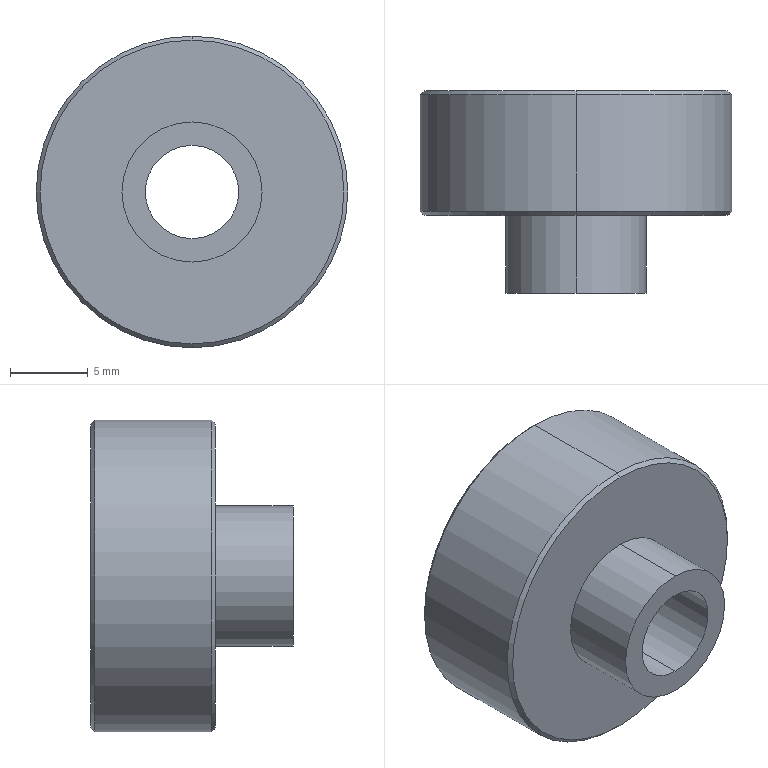Part | STEP file | BCC3 H14_12 | 1 solid | 13 faces | box 20 x 13 x 20 mm | volume 2460 mm3 | cylinder 6 | cone 4 | plane 3 | commonest cylinder face diameters 6 x2 9 x2 20 x2
STEP:
#1=CARTESIAN_POINT('',(0.,0.,0.));
#2=DIRECTION('',(0.,0.,1.));
#3=DIRECTION('',(1.,0.,0.));
#4=AXIS2_PLACEMENT_3D('',#1,#2,#3);
#5=CARTESIAN_POINT('',(0.,8.,9.75));
#6=VERTEX_POINT('',#5);
#7=CARTESIAN_POINT('',(0.,8.,-9.75));
#8=VERTEX_POINT('',#7);
#9=CARTESIAN_POINT('',(0.,8.,0.));
#10=DIRECTION('',(0.,1.,0.));
#11=DIRECTION('',(0.,0.,1.));
#12=AXIS2_PLACEMENT_3D('',#9,#10,#11);
#13=CIRCLE('',#12,9.75);
#14=CARTESIAN_POINT('',(0.,8.,0.));
#15=DIRECTION('',(0.,-1.,0.));
#16=DIRECTION('',(0.,0.,-1.));
#17=AXIS2_PLACEMENT_3D('',#14,#15,#16);
#18=CONICAL_SURFACE('',#17,9.75,0.7854);
#19=CARTESIAN_POINT('',(3.142,0.));
#20=DIRECTION('',(-1.,0.));
#21=VECTOR('',#20,1.);
#22=LINE('',#19,#21);
#23=(GEOMETRIC_REPRESENTATION_CONTEXT(2)PARAMETRIC_REPRESENTATION_CONTEXT()REPRESENTATION_CONTEXT('',''));
#24=DEFINITIONAL_REPRESENTATION('',(#22),#23);
#25=PCURVE('',#18,#24);
#26=CARTESIAN_POINT('',(0.,8.,0.));
#27=DIRECTION('',(0.,1.,0.));
#28=DIRECTION('',(0.,0.,1.));
#29=AXIS2_PLACEMENT_3D('',#26,#27,#28);
#30=PLANE('',#29);
#31=CARTESIAN_POINT('',(0.,0.));
#32=DIRECTION('',(1.,0.));
#33=AXIS2_PLACEMENT_2D('',#31,#32);
#34=CIRCLE('',#33,9.75);
#35=(GEOMETRIC_REPRESENTATION_CONTEXT(2)PARAMETRIC_REPRESENTATION_CONTEXT()REPRESENTATION_CONTEXT('',''));
#36=DEFINITIONAL_REPRESENTATION('',(#34),#35);
#37=PCURVE('',#30,#36);
#38=SURFACE_CURVE('',#13,(#25,#37),.PCURVE_S1.);
#39=EDGE_CURVE('',#6,#8,#38,.T.);
#40=ORIENTED_EDGE('',*,*,#39,.F.);
#41=CARTESIAN_POINT('',(0.,7.75,10.));
#42=VERTEX_POINT('',#41);
#43=CARTESIAN_POINT('',(0.,8.,9.75));
#44=DIRECTION('',(0.,-0.7071,0.7071));
#45=VECTOR('',#44,1.);
#46=LINE('',#43,#45);
#47=CARTESIAN_POINT('',(3.142,0.));
#48=DIRECTION('',(0.,1.));
#49=VECTOR('',#48,1.);
#50=LINE('',#47,#49);
#51=(GEOMETRIC_REPRESENTATION_CONTEXT(2)PARAMETRIC_REPRESENTATION_CONTEXT()REPRESENTATION_CONTEXT('',''));
#52=DEFINITIONAL_REPRESENTATION('',(#50),#51);
#53=PCURVE('',#18,#52);
#54=CARTESIAN_POINT('',(0.,8.,0.));
#55=DIRECTION('',(0.,-1.,0.));
#56=DIRECTION('',(0.,0.,-1.));
#57=AXIS2_PLACEMENT_3D('',#54,#55,#56);
#58=CONICAL_SURFACE('',#57,9.75,0.7854);
#59=CARTESIAN_POINT('',(3.142,0.));
#60=DIRECTION('',(0.,1.));
#61=VECTOR('',#60,1.);
#62=LINE('',#59,#61);
#63=(GEOMETRIC_REPRESENTATION_CONTEXT(2)PARAMETRIC_REPRESENTATION_CONTEXT()REPRESENTATION_CONTEXT('',''));
#64=DEFINITIONAL_REPRESENTATION('',(#62),#63);
#65=PCURVE('',#58,#64);
#66=SURFACE_CURVE('',#46,(#53,#65),.PCURVE_S1.);
#67=EDGE_CURVE('',#6,#42,#66,.T.);
#68=ORIENTED_EDGE('',*,*,#67,.T.);
#69=CARTESIAN_POINT('',(0.,7.75,-10.));
#70=VERTEX_POINT('',#69);
#71=CARTESIAN_POINT('',(0.,7.75,0.));
#72=DIRECTION('',(0.,-1.,0.));
#73=DIRECTION('',(0.,0.,1.));
#74=AXIS2_PLACEMENT_3D('',#71,#72,#73);
#75=CIRCLE('',#74,10.);
#76=CARTESIAN_POINT('',(-3.142,0.25));
#77=DIRECTION('',(1.,0.));
#78=VECTOR('',#77,1.);
#79=LINE('',#76,#78);
#80=(GEOMETRIC_REPRESENTATION_CONTEXT(2)PARAMETRIC_REPRESENTATION_CONTEXT()REPRESENTATION_CONTEXT('',''));
#81=DEFINITIONAL_REPRESENTATION('',(#79),#80);
#82=PCURVE('',#18,#81);
#83=CARTESIAN_POINT('',(0.,8.,0.));
#84=DIRECTION('',(0.,-1.,0.));
#85=DIRECTION('',(0.,0.,-1.));
#86=AXIS2_PLACEMENT_3D('',#83,#84,#85);
#87=CYLINDRICAL_SURFACE('',#86,10.);
#88=CARTESIAN_POINT('',(-3.142,0.25));
#89=DIRECTION('',(1.,0.));
#90=VECTOR('',#89,1.);
#91=LINE('',#88,#90);
#92=(GEOMETRIC_REPRESENTATION_CONTEXT(2)PARAMETRIC_REPRESENTATION_CONTEXT()REPRESENTATION_CONTEXT('',''));
#93=DEFINITIONAL_REPRESENTATION('',(#91),#92);
#94=PCURVE('',#87,#93);
#95=SURFACE_CURVE('',#75,(#82,#94),.PCURVE_S1.);
#96=EDGE_CURVE('',#70,#42,#95,.T.);
#97=ORIENTED_EDGE('',*,*,#96,.F.);
#98=CARTESIAN_POINT('',(0.,8.,-9.75));
#99=DIRECTION('',(0.,-0.7071,-0.7071));
#100=VECTOR('',#99,1.);
#101=LINE('',#98,#100);
#102=CARTESIAN_POINT('',(0.,0.));
#103=DIRECTION('',(0.,1.));
#104=VECTOR('',#103,1.);
#105=LINE('',#102,#104);
#106=(GEOMETRIC_REPRESENTATION_CONTEXT(2)PARAMETRIC_REPRESENTATION_CONTEXT()REPRESENTATION_CONTEXT('',''));
#107=DEFINITIONAL_REPRESENTATION('',(#105),#106);
#108=PCURVE('',#18,#107);
#109=CARTESIAN_POINT('',(6.283,0.));
#110=DIRECTION('',(0.,1.));
#111=VECTOR('',#110,1.);
#112=LINE('',#109,#111);
#113=(GEOMETRIC_REPRESENTATION_CONTEXT(2)PARAMETRIC_REPRESENTATION_CONTEXT()REPRESENTATION_CONTEXT('',''));
#114=DEFINITIONAL_REPRESENTATION('',(#112),#113);
#115=PCURVE('',#58,#114);
#116=SURFACE_CURVE('',#101,(#108,#115),.PCURVE_S1.);
#117=EDGE_CURVE('',#8,#70,#116,.T.);
#118=ORIENTED_EDGE('',*,*,#117,.F.);
#119=EDGE_LOOP('',(#40,#68,#97,#118));
#120=FACE_BOUND('',#119,.T.);
#121=ADVANCED_FACE('',(#120),#18,.T.);
#122=CARTESIAN_POINT('',(0.,0.,-9.75));
#123=VERTEX_POINT('',#122);
#124=CARTESIAN_POINT('',(0.,0.,9.75));
#125=VERTEX_POINT('',#124);
#126=CARTESIAN_POINT('',(0.,0.,0.));
#127=DIRECTION('',(0.,-1.,0.));
#128=DIRECTION('',(0.,0.,1.));
#129=AXIS2_PLACEMENT_3D('',#126,#127,#128);
#130=CIRCLE('',#129,9.75);
#131=CARTESIAN_POINT('',(0.,0.25,0.));
#132=DIRECTION('',(0.,1.,0.));
#133=DIRECTION('',(0.,0.,1.));
#134=AXIS2_PLACEMENT_3D('',#131,#132,#133);
#135=CONICAL_SURFACE('',#134,10.,0.7854);
#136=CARTESIAN_POINT('',(6.283,-0.25));
#137=DIRECTION('',(-1.,0.));
#138=VECTOR('',#137,1.);
#139=LINE('',#136,#138);
#140=(GEOMETRIC_REPRESENTATION_CONTEXT(2)PARAMETRIC_REPRESENTATION_CONTEXT()REPRESENTATION_CONTEXT('',''));
#141=DEFINITIONAL_REPRESENTATION('',(#139),#140);
#142=PCURVE('',#135,#141);
#143=CARTESIAN_POINT('',(0.,0.,0.));
#144=DIRECTION('',(0.,1.,0.));
#145=DIRECTION('',(0.,0.,1.));
#146=AXIS2_PLACEMENT_3D('',#143,#144,#145);
#147=PLANE('',#146);
#148=CARTESIAN_POINT('',(9.75,0.));
#149=CARTESIAN_POINT('',(9.75,-16.887));
#150=CARTESIAN_POINT('',(-4.875,-8.444));
#151=CARTESIAN_POINT('',(-19.5,0.));
#152=CARTESIAN_POINT('',(-4.875,8.444));
#153=CARTESIAN_POINT('',(9.75,16.887));
#154=CARTESIAN_POINT('',(9.75,0.));
#155=(BOUNDED_CURVE()B_SPLINE_CURVE(2,(#148,#149,#150,#151,#152,#153,#154),.UNSPECIFIED.,.T.,.F.)B_SPLINE_CURVE_WITH_KNOTS((1,2,2,2,2,1),(-2.094,0.,2.094,4.189,6.283,8.378),.UNSPECIFIED.)CURVE()GEOMETRIC_REPRESENTATION_ITEM()RATIONAL_B_SPLINE_CURVE((1.,0.5,1.,0.5,1.,0.5,1.))REPRESENTATION_ITEM(''));
#156=(GEOMETRIC_REPRESENTATION_CONTEXT(2)PARAMETRIC_REPRESENTATION_CONTEXT()REPRESENTATION_CONTEXT('',''));
#157=DEFINITIONAL_REPRESENTATION('',(#155),#156);
#158=PCURVE('',#147,#157);
#159=SURFACE_CURVE('',#130,(#142,#158),.PCURVE_S1.);
#160=EDGE_CURVE('',#123,#125,#159,.T.);
#161=ORIENTED_EDGE('',*,*,#160,.F.);
#162=CARTESIAN_POINT('',(0.,0.25,-10.));
#163=VERTEX_POINT('',#162);
#164=CARTESIAN_POINT('',(0.,0.25,-10.));
#165=DIRECTION('',(0.,0.7071,-0.7071));
#166=VECTOR('',#165,1.);
#167=LINE('',#164,#166);
#168=CARTESIAN_POINT('',(3.142,0.));
#169=DIRECTION('',(0.,1.));
#170=VECTOR('',#169,1.);
#171=LINE('',#168,#170);
#172=(GEOMETRIC_REPRESENTATION_CONTEXT(2)PARAMETRIC_REPRESENTATION_CONTEXT()REPRESENTATION_CONTEXT('',''));
#173=DEFINITIONAL_REPRESENTATION('',(#171),#172);
#174=PCURVE('',#135,#173);
#175=CARTESIAN_POINT('',(0.,0.25,0.));
#176=DIRECTION('',(0.,1.,0.));
#177=DIRECTION('',(0.,0.,1.));
#178=AXIS2_PLACEMENT_3D('',#175,#176,#177);
#179=CONICAL_SURFACE('',#178,10.,0.7854);
#180=CARTESIAN_POINT('',(3.142,0.));
#181=DIRECTION('',(0.,1.));
#182=VECTOR('',#181,1.);
#183=LINE('',#180,#182);
#184=(GEOMETRIC_REPRESENTATION_CONTEXT(2)PARAMETRIC_REPRESENTATION_CONTEXT()REPRESENTATION_CONTEXT('',''));
#185=DEFINITIONAL_REPRESENTATION('',(#183),#184);
#186=PCURVE('',#179,#185);
#187=SURFACE_CURVE('',#167,(#174,#186),.PCURVE_S1.);
#188=EDGE_CURVE('',#123,#163,#187,.T.);
#189=ORIENTED_EDGE('',*,*,#188,.T.);
#190=CARTESIAN_POINT('',(0.,0.25,10.));
#191=VERTEX_POINT('',#190);
#192=CARTESIAN_POINT('',(0.,0.25,0.));
#193=DIRECTION('',(0.,1.,0.));
#194=DIRECTION('',(0.,0.,1.));
#195=AXIS2_PLACEMENT_3D('',#192,#193,#194);
#196=CIRCLE('',#195,10.);
#197=CARTESIAN_POINT('',(0.,0.));
#198=DIRECTION('',(1.,0.));
#199=VECTOR('',#198,1.);
#200=LINE('',#197,#199);
#201=(GEOMETRIC_REPRESENTATION_CONTEXT(2)PARAMETRIC_REPRESENTATION_CONTEXT()REPRESENTATION_CONTEXT('',''));
#202=DEFINITIONAL_REPRESENTATION('',(#200),#201);
#203=PCURVE('',#135,#202);
#204=CARTESIAN_POINT('',(3.142,7.75));
#205=DIRECTION('',(-1.,0.));
#206=VECTOR('',#205,1.);
#207=LINE('',#204,#206);
#208=(GEOMETRIC_REPRESENTATION_CONTEXT(2)PARAMETRIC_REPRESENTATION_CONTEXT()REPRESENTATION_CONTEXT('',''));
#209=DEFINITIONAL_REPRESENTATION('',(#207),#208);
#210=PCURVE('',#87,#209);
#211=SURFACE_CURVE('',#196,(#203,#210),.PCURVE_S1.);
#212=EDGE_CURVE('',#191,#163,#211,.T.);
#213=ORIENTED_EDGE('',*,*,#212,.F.);
#214=CARTESIAN_POINT('',(0.,0.25,10.));
#215=DIRECTION('',(0.,0.7071,0.7071));
#216=VECTOR('',#215,1.);
#217=LINE('',#214,#216);
#218=CARTESIAN_POINT('',(0.,0.));
#219=DIRECTION('',(0.,1.));
#220=VECTOR('',#219,1.);
#221=LINE('',#218,#220);
#222=(GEOMETRIC_REPRESENTATION_CONTEXT(2)PARAMETRIC_REPRESENTATION_CONTEXT()REPRESENTATION_CONTEXT('',''));
#223=DEFINITIONAL_REPRESENTATION('',(#221),#222);
#224=PCURVE('',#135,#223);
#225=CARTESIAN_POINT('',(6.283,0.));
#226=DIRECTION('',(0.,1.));
#227=VECTOR('',#226,1.);
#228=LINE('',#225,#227);
#229=(GEOMETRIC_REPRESENTATION_CONTEXT(2)PARAMETRIC_REPRESENTATION_CONTEXT()REPRESENTATION_CONTEXT('',''));
#230=DEFINITIONAL_REPRESENTATION('',(#228),#229);
#231=PCURVE('',#179,#230);
#232=SURFACE_CURVE('',#217,(#224,#231),.PCURVE_S1.);
#233=EDGE_CURVE('',#125,#191,#232,.T.);
#234=ORIENTED_EDGE('',*,*,#233,.F.);
#235=EDGE_LOOP('',(#161,#189,#213,#234));
#236=FACE_BOUND('',#235,.T.);
#237=ADVANCED_FACE('',(#236),#135,.T.);
#238=CARTESIAN_POINT('',(0.,-5.,-4.5));
#239=VERTEX_POINT('',#238);
#240=CARTESIAN_POINT('',(0.,-5.,4.5));
#241=VERTEX_POINT('',#240);
#242=CARTESIAN_POINT('',(0.,-5.,0.));
#243=DIRECTION('',(0.,-1.,0.));
#244=DIRECTION('',(0.,0.,-1.));
#245=AXIS2_PLACEMENT_3D('',#242,#243,#244);
#246=CIRCLE('',#245,4.5);
#247=CARTESIAN_POINT('',(0.,-5.,0.));
#248=DIRECTION('',(0.,1.,0.));
#249=DIRECTION('',(0.,0.,1.));
#250=AXIS2_PLACEMENT_3D('',#247,#248,#249);
#251=CYLINDRICAL_SURFACE('',#250,4.5);
#252=CARTESIAN_POINT('',(3.142,0.));
#253=DIRECTION('',(-1.,0.));
#254=VECTOR('',#253,1.);
#255=LINE('',#252,#254);
#256=(GEOMETRIC_REPRESENTATION_CONTEXT(2)PARAMETRIC_REPRESENTATION_CONTEXT()REPRESENTATION_CONTEXT('',''));
#257=DEFINITIONAL_REPRESENTATION('',(#255),#256);
#258=PCURVE('',#251,#257);
#259=CARTESIAN_POINT('',(0.,-5.,0.));
#260=DIRECTION('',(0.,-1.,0.));
#261=DIRECTION('',(0.,0.,-1.));
#262=AXIS2_PLACEMENT_3D('',#259,#260,#261);
#263=PLANE('',#262);
#264=CARTESIAN_POINT('',(0.,0.));
#265=DIRECTION('',(1.,0.));
#266=AXIS2_PLACEMENT_2D('',#264,#265);
#267=CIRCLE('',#266,4.5);
#268=(GEOMETRIC_REPRESENTATION_CONTEXT(2)PARAMETRIC_REPRESENTATION_CONTEXT()REPRESENTATION_CONTEXT('',''));
#269=DEFINITIONAL_REPRESENTATION('',(#267),#268);
#270=PCURVE('',#263,#269);
#271=SURFACE_CURVE('',#246,(#258,#270),.PCURVE_S1.);
#272=EDGE_CURVE('',#239,#241,#271,.T.);
#273=ORIENTED_EDGE('',*,*,#272,.F.);
#274=CARTESIAN_POINT('',(0.,0.,-4.5));
#275=VERTEX_POINT('',#274);
#276=CARTESIAN_POINT('',(0.,-5.,-4.5));
#277=DIRECTION('',(0.,1.,0.));
#278=VECTOR('',#277,1.);
#279=LINE('',#276,#278);
#280=CARTESIAN_POINT('',(3.142,0.));
#281=DIRECTION('',(0.,1.));
#282=VECTOR('',#281,1.);
#283=LINE('',#280,#282);
#284=(GEOMETRIC_REPRESENTATION_CONTEXT(2)PARAMETRIC_REPRESENTATION_CONTEXT()REPRESENTATION_CONTEXT('',''));
#285=DEFINITIONAL_REPRESENTATION('',(#283),#284);
#286=PCURVE('',#251,#285);
#287=CARTESIAN_POINT('',(0.,-5.,0.));
#288=DIRECTION('',(0.,1.,0.));
#289=DIRECTION('',(0.,0.,1.));
#290=AXIS2_PLACEMENT_3D('',#287,#288,#289);
#291=CYLINDRICAL_SURFACE('',#290,4.5);
#292=CARTESIAN_POINT('',(3.142,0.));
#293=DIRECTION('',(0.,1.));
#294=VECTOR('',#293,1.);
#295=LINE('',#292,#294);
#296=(GEOMETRIC_REPRESENTATION_CONTEXT(2)PARAMETRIC_REPRESENTATION_CONTEXT()REPRESENTATION_CONTEXT('',''));
#297=DEFINITIONAL_REPRESENTATION('',(#295),#296);
#298=PCURVE('',#291,#297);
#299=SURFACE_CURVE('',#279,(#286,#298),.PCURVE_S1.);
#300=EDGE_CURVE('',#239,#275,#299,.T.);
#301=ORIENTED_EDGE('',*,*,#300,.T.);
#302=CARTESIAN_POINT('',(0.,0.,4.5));
#303=VERTEX_POINT('',#302);
#304=CARTESIAN_POINT('',(0.,0.,0.));
#305=DIRECTION('',(0.,-1.,0.));
#306=DIRECTION('',(0.,0.,1.));
#307=AXIS2_PLACEMENT_3D('',#304,#305,#306);
#308=CIRCLE('',#307,4.5);
#309=CARTESIAN_POINT('',(6.283,5.));
#310=DIRECTION('',(-1.,0.));
#311=VECTOR('',#310,1.);
#312=LINE('',#309,#311);
#313=(GEOMETRIC_REPRESENTATION_CONTEXT(2)PARAMETRIC_REPRESENTATION_CONTEXT()REPRESENTATION_CONTEXT('',''));
#314=DEFINITIONAL_REPRESENTATION('',(#312),#313);
#315=PCURVE('',#251,#314);
#316=CARTESIAN_POINT('',(4.5,0.));
#317=CARTESIAN_POINT('',(4.5,-7.794));
#318=CARTESIAN_POINT('',(-2.25,-3.897));
#319=CARTESIAN_POINT('',(-9.,0.));
#320=CARTESIAN_POINT('',(-2.25,3.897));
#321=CARTESIAN_POINT('',(4.5,7.794));
#322=CARTESIAN_POINT('',(4.5,0.));
#323=(BOUNDED_CURVE()B_SPLINE_CURVE(2,(#316,#317,#318,#319,#320,#321,#322),.UNSPECIFIED.,.T.,.F.)B_SPLINE_CURVE_WITH_KNOTS((1,2,2,2,2,1),(-2.094,0.,2.094,4.189,6.283,8.378),.UNSPECIFIED.)CURVE()GEOMETRIC_REPRESENTATION_ITEM()RATIONAL_B_SPLINE_CURVE((1.,0.5,1.,0.5,1.,0.5,1.))REPRESENTATION_ITEM(''));
#324=(GEOMETRIC_REPRESENTATION_CONTEXT(2)PARAMETRIC_REPRESENTATION_CONTEXT()REPRESENTATION_CONTEXT('',''));
#325=DEFINITIONAL_REPRESENTATION('',(#323),#324);
#326=PCURVE('',#147,#325);
#327=SURFACE_CURVE('',#308,(#315,#326),.PCURVE_S1.);
#328=EDGE_CURVE('',#275,#303,#327,.T.);
#329=ORIENTED_EDGE('',*,*,#328,.T.);
#330=CARTESIAN_POINT('',(0.,-5.,4.5));
#331=DIRECTION('',(0.,1.,0.));
#332=VECTOR('',#331,1.);
#333=LINE('',#330,#332);
#334=CARTESIAN_POINT('',(0.,0.));
#335=DIRECTION('',(0.,1.));
#336=VECTOR('',#335,1.);
#337=LINE('',#334,#336);
#338=(GEOMETRIC_REPRESENTATION_CONTEXT(2)PARAMETRIC_REPRESENTATION_CONTEXT()REPRESENTATION_CONTEXT('',''));
#339=DEFINITIONAL_REPRESENTATION('',(#337),#338);
#340=PCURVE('',#251,#339);
#341=CARTESIAN_POINT('',(6.283,0.));
#342=DIRECTION('',(0.,1.));
#343=VECTOR('',#342,1.);
#344=LINE('',#341,#343);
#345=(GEOMETRIC_REPRESENTATION_CONTEXT(2)PARAMETRIC_REPRESENTATION_CONTEXT()REPRESENTATION_CONTEXT('',''));
#346=DEFINITIONAL_REPRESENTATION('',(#344),#345);
#347=PCURVE('',#291,#346);
#348=SURFACE_CURVE('',#333,(#340,#347),.PCURVE_S1.);
#349=EDGE_CURVE('',#241,#303,#348,.T.);
#350=ORIENTED_EDGE('',*,*,#349,.F.);
#351=EDGE_LOOP('',(#273,#301,#329,#350));
#352=FACE_BOUND('',#351,.T.);
#353=ADVANCED_FACE('',(#352),#251,.T.);
#354=CARTESIAN_POINT('',(0.,8.,-3.));
#355=VERTEX_POINT('',#354);
#356=CARTESIAN_POINT('',(0.,-5.,-3.));
#357=VERTEX_POINT('',#356);
#358=CARTESIAN_POINT('',(0.,8.,-3.));
#359=DIRECTION('',(0.,-1.,0.));
#360=VECTOR('',#359,1.);
#361=LINE('',#358,#360);
#362=CARTESIAN_POINT('',(0.,8.,0.));
#363=DIRECTION('',(0.,-1.,0.));
#364=DIRECTION('',(0.,0.,-1.));
#365=AXIS2_PLACEMENT_3D('',#362,#363,#364);
#366=CYLINDRICAL_SURFACE('',#365,3.);
#367=CARTESIAN_POINT('',(6.283,0.));
#368=DIRECTION('',(0.,1.));
#369=VECTOR('',#368,1.);
#370=LINE('',#367,#369);
#371=(GEOMETRIC_REPRESENTATION_CONTEXT(2)PARAMETRIC_REPRESENTATION_CONTEXT()REPRESENTATION_CONTEXT('',''));
#372=DEFINITIONAL_REPRESENTATION('',(#370),#371);
#373=PCURVE('',#366,#372);
#374=CARTESIAN_POINT('',(0.,8.,0.));
#375=DIRECTION('',(0.,-1.,0.));
#376=DIRECTION('',(0.,0.,-1.));
#377=AXIS2_PLACEMENT_3D('',#374,#375,#376);
#378=CYLINDRICAL_SURFACE('',#377,3.);
#379=CARTESIAN_POINT('',(0.,0.));
#380=DIRECTION('',(0.,1.));
#381=VECTOR('',#380,1.);
#382=LINE('',#379,#381);
#383=(GEOMETRIC_REPRESENTATION_CONTEXT(2)PARAMETRIC_REPRESENTATION_CONTEXT()REPRESENTATION_CONTEXT('',''));
#384=DEFINITIONAL_REPRESENTATION('',(#382),#383);
#385=PCURVE('',#378,#384);
#386=SURFACE_CURVE('',#361,(#373,#385),.PCURVE_S1.);
#387=EDGE_CURVE('',#355,#357,#386,.T.);
#388=ORIENTED_EDGE('',*,*,#387,.T.);
#389=CARTESIAN_POINT('',(0.,-5.,3.));
#390=VERTEX_POINT('',#389);
#391=CARTESIAN_POINT('',(0.,-5.,0.));
#392=DIRECTION('',(0.,-1.,0.));
#393=DIRECTION('',(0.,0.,-1.));
#394=AXIS2_PLACEMENT_3D('',#391,#392,#393);
#395=CIRCLE('',#394,3.);
#396=CARTESIAN_POINT('',(0.,13.));
#397=DIRECTION('',(1.,0.));
#398=VECTOR('',#397,1.);
#399=LINE('',#396,#398);
#400=(GEOMETRIC_REPRESENTATION_CONTEXT(2)PARAMETRIC_REPRESENTATION_CONTEXT()REPRESENTATION_CONTEXT('',''));
#401=DEFINITIONAL_REPRESENTATION('',(#399),#400);
#402=PCURVE('',#366,#401);
#403=CARTESIAN_POINT('',(0.,0.));
#404=DIRECTION('',(1.,0.));
#405=AXIS2_PLACEMENT_2D('',#403,#404);
#406=CIRCLE('',#405,3.);
#407=(GEOMETRIC_REPRESENTATION_CONTEXT(2)PARAMETRIC_REPRESENTATION_CONTEXT()REPRESENTATION_CONTEXT('',''));
#408=DEFINITIONAL_REPRESENTATION('',(#406),#407);
#409=PCURVE('',#263,#408);
#410=SURFACE_CURVE('',#395,(#402,#409),.PCURVE_S1.);
#411=EDGE_CURVE('',#390,#357,#410,.T.);
#412=ORIENTED_EDGE('',*,*,#411,.F.);
#413=CARTESIAN_POINT('',(0.,8.,3.));
#414=VERTEX_POINT('',#413);
#415=CARTESIAN_POINT('',(0.,8.,3.));
#416=DIRECTION('',(0.,-1.,0.));
#417=VECTOR('',#416,1.);
#418=LINE('',#415,#417);
#419=CARTESIAN_POINT('',(3.142,0.));
#420=DIRECTION('',(0.,1.));
#421=VECTOR('',#420,1.);
#422=LINE('',#419,#421);
#423=(GEOMETRIC_REPRESENTATION_CONTEXT(2)PARAMETRIC_REPRESENTATION_CONTEXT()REPRESENTATION_CONTEXT('',''));
#424=DEFINITIONAL_REPRESENTATION('',(#422),#423);
#425=PCURVE('',#366,#424);
#426=CARTESIAN_POINT('',(3.142,0.));
#427=DIRECTION('',(0.,1.));
#428=VECTOR('',#427,1.);
#429=LINE('',#426,#428);
#430=(GEOMETRIC_REPRESENTATION_CONTEXT(2)PARAMETRIC_REPRESENTATION_CONTEXT()REPRESENTATION_CONTEXT('',''));
#431=DEFINITIONAL_REPRESENTATION('',(#429),#430);
#432=PCURVE('',#378,#431);
#433=SURFACE_CURVE('',#418,(#425,#432),.PCURVE_S1.);
#434=EDGE_CURVE('',#414,#390,#433,.T.);
#435=ORIENTED_EDGE('',*,*,#434,.F.);
#436=CARTESIAN_POINT('',(0.,8.,0.));
#437=DIRECTION('',(0.,1.,0.));
#438=DIRECTION('',(0.,0.,1.));
#439=AXIS2_PLACEMENT_3D('',#436,#437,#438);
#440=CIRCLE('',#439,3.);
#441=CARTESIAN_POINT('',(9.425,0.));
#442=DIRECTION('',(-1.,0.));
#443=VECTOR('',#442,1.);
#444=LINE('',#441,#443);
#445=(GEOMETRIC_REPRESENTATION_CONTEXT(2)PARAMETRIC_REPRESENTATION_CONTEXT()REPRESENTATION_CONTEXT('',''));
#446=DEFINITIONAL_REPRESENTATION('',(#444),#445);
#447=PCURVE('',#366,#446);
#448=CARTESIAN_POINT('',(0.,0.));
#449=DIRECTION('',(1.,0.));
#450=AXIS2_PLACEMENT_2D('',#448,#449);
#451=CIRCLE('',#450,3.);
#452=(GEOMETRIC_REPRESENTATION_CONTEXT(2)PARAMETRIC_REPRESENTATION_CONTEXT()REPRESENTATION_CONTEXT('',''));
#453=DEFINITIONAL_REPRESENTATION('',(#451),#452);
#454=PCURVE('',#30,#453);
#455=SURFACE_CURVE('',#440,(#447,#454),.PCURVE_S1.);
#456=EDGE_CURVE('',#355,#414,#455,.T.);
#457=ORIENTED_EDGE('',*,*,#456,.F.);
#458=EDGE_LOOP('',(#388,#412,#435,#457));
#459=FACE_BOUND('',#458,.F.);
#460=ADVANCED_FACE('',(#459),#366,.F.);
#461=ORIENTED_EDGE('',*,*,#96,.T.);
#462=CARTESIAN_POINT('',(0.,8.,10.));
#463=DIRECTION('',(0.,-1.,0.));
#464=VECTOR('',#463,1.);
#465=LINE('',#462,#464);
#466=CARTESIAN_POINT('',(3.142,0.));
#467=DIRECTION('',(0.,1.));
#468=VECTOR('',#467,1.);
#469=LINE('',#466,#468);
#470=(GEOMETRIC_REPRESENTATION_CONTEXT(2)PARAMETRIC_REPRESENTATION_CONTEXT()REPRESENTATION_CONTEXT('',''));
#471=DEFINITIONAL_REPRESENTATION('',(#469),#470);
#472=PCURVE('',#87,#471);
#473=CARTESIAN_POINT('',(0.,8.,0.));
#474=DIRECTION('',(0.,-1.,0.));
#475=DIRECTION('',(0.,0.,-1.));
#476=AXIS2_PLACEMENT_3D('',#473,#474,#475);
#477=CYLINDRICAL_SURFACE('',#476,10.);
#478=CARTESIAN_POINT('',(3.142,0.));
#479=DIRECTION('',(0.,1.));
#480=VECTOR('',#479,1.);
#481=LINE('',#478,#480);
#482=(GEOMETRIC_REPRESENTATION_CONTEXT(2)PARAMETRIC_REPRESENTATION_CONTEXT()REPRESENTATION_CONTEXT('',''));
#483=DEFINITIONAL_REPRESENTATION('',(#481),#482);
#484=PCURVE('',#477,#483);
#485=SURFACE_CURVE('',#465,(#472,#484),.PCURVE_S1.);
#486=EDGE_CURVE('',#42,#191,#485,.T.);
#487=ORIENTED_EDGE('',*,*,#486,.T.);
#488=ORIENTED_EDGE('',*,*,#212,.T.);
#489=CARTESIAN_POINT('',(0.,8.,-10.));
#490=DIRECTION('',(0.,-1.,0.));
#491=VECTOR('',#490,1.);
#492=LINE('',#489,#491);
#493=CARTESIAN_POINT('',(0.,0.));
#494=DIRECTION('',(0.,1.));
#495=VECTOR('',#494,1.);
#496=LINE('',#493,#495);
#497=(GEOMETRIC_REPRESENTATION_CONTEXT(2)PARAMETRIC_REPRESENTATION_CONTEXT()REPRESENTATION_CONTEXT('',''));
#498=DEFINITIONAL_REPRESENTATION('',(#496),#497);
#499=PCURVE('',#87,#498);
#500=CARTESIAN_POINT('',(6.283,0.));
#501=DIRECTION('',(0.,1.));
#502=VECTOR('',#501,1.);
#503=LINE('',#500,#502);
#504=(GEOMETRIC_REPRESENTATION_CONTEXT(2)PARAMETRIC_REPRESENTATION_CONTEXT()REPRESENTATION_CONTEXT('',''));
#505=DEFINITIONAL_REPRESENTATION('',(#503),#504);
#506=PCURVE('',#477,#505);
#507=SURFACE_CURVE('',#492,(#499,#506),.PCURVE_S1.);
#508=EDGE_CURVE('',#70,#163,#507,.T.);
#509=ORIENTED_EDGE('',*,*,#508,.F.);
#510=EDGE_LOOP('',(#461,#487,#488,#509));
#511=FACE_BOUND('',#510,.T.);
#512=ADVANCED_FACE('',(#511),#87,.T.);
#513=CARTESIAN_POINT('',(0.,0.,0.));
#514=DIRECTION('',(0.,-1.,0.));
#515=DIRECTION('',(0.,0.,1.));
#516=AXIS2_PLACEMENT_3D('',#513,#514,#515);
#517=CIRCLE('',#516,9.75);
#518=CARTESIAN_POINT('',(9.75,0.));
#519=CARTESIAN_POINT('',(9.75,-16.887));
#520=CARTESIAN_POINT('',(-4.875,-8.444));
#521=CARTESIAN_POINT('',(-19.5,0.));
#522=CARTESIAN_POINT('',(-4.875,8.444));
#523=CARTESIAN_POINT('',(9.75,16.887));
#524=CARTESIAN_POINT('',(9.75,0.));
#525=(BOUNDED_CURVE()B_SPLINE_CURVE(2,(#518,#519,#520,#521,#522,#523,#524),.UNSPECIFIED.,.T.,.F.)B_SPLINE_CURVE_WITH_KNOTS((1,2,2,2,2,1),(-2.094,0.,2.094,4.189,6.283,8.378),.UNSPECIFIED.)CURVE()GEOMETRIC_REPRESENTATION_ITEM()RATIONAL_B_SPLINE_CURVE((1.,0.5,1.,0.5,1.,0.5,1.))REPRESENTATION_ITEM(''));
#526=(GEOMETRIC_REPRESENTATION_CONTEXT(2)PARAMETRIC_REPRESENTATION_CONTEXT()REPRESENTATION_CONTEXT('',''));
#527=DEFINITIONAL_REPRESENTATION('',(#525),#526);
#528=PCURVE('',#147,#527);
#529=CARTESIAN_POINT('',(6.283,-0.25));
#530=DIRECTION('',(-1.,0.));
#531=VECTOR('',#530,1.);
#532=LINE('',#529,#531);
#533=(GEOMETRIC_REPRESENTATION_CONTEXT(2)PARAMETRIC_REPRESENTATION_CONTEXT()REPRESENTATION_CONTEXT('',''));
#534=DEFINITIONAL_REPRESENTATION('',(#532),#533);
#535=PCURVE('',#179,#534);
#536=SURFACE_CURVE('',#517,(#528,#535),.PCURVE_S1.);
#537=EDGE_CURVE('',#125,#123,#536,.T.);
#538=ORIENTED_EDGE('',*,*,#537,.T.);
#539=ORIENTED_EDGE('',*,*,#160,.T.);
#540=EDGE_LOOP('',(#538,#539));
#541=FACE_BOUND('',#540,.T.);
#542=CARTESIAN_POINT('',(0.,0.,0.));
#543=DIRECTION('',(0.,-1.,0.));
#544=DIRECTION('',(0.,0.,1.));
#545=AXIS2_PLACEMENT_3D('',#542,#543,#544);
#546=CIRCLE('',#545,4.5);
#547=CARTESIAN_POINT('',(4.5,0.));
#548=CARTESIAN_POINT('',(4.5,-7.794));
#549=CARTESIAN_POINT('',(-2.25,-3.897));
#550=CARTESIAN_POINT('',(-9.,0.));
#551=CARTESIAN_POINT('',(-2.25,3.897));
#552=CARTESIAN_POINT('',(4.5,7.794));
#553=CARTESIAN_POINT('',(4.5,0.));
#554=(BOUNDED_CURVE()B_SPLINE_CURVE(2,(#547,#548,#549,#550,#551,#552,#553),.UNSPECIFIED.,.T.,.F.)B_SPLINE_CURVE_WITH_KNOTS((1,2,2,2,2,1),(-2.094,0.,2.094,4.189,6.283,8.378),.UNSPECIFIED.)CURVE()GEOMETRIC_REPRESENTATION_ITEM()RATIONAL_B_SPLINE_CURVE((1.,0.5,1.,0.5,1.,0.5,1.))REPRESENTATION_ITEM(''));
#555=(GEOMETRIC_REPRESENTATION_CONTEXT(2)PARAMETRIC_REPRESENTATION_CONTEXT()REPRESENTATION_CONTEXT('',''));
#556=DEFINITIONAL_REPRESENTATION('',(#554),#555);
#557=PCURVE('',#147,#556);
#558=CARTESIAN_POINT('',(6.283,5.));
#559=DIRECTION('',(-1.,0.));
#560=VECTOR('',#559,1.);
#561=LINE('',#558,#560);
#562=(GEOMETRIC_REPRESENTATION_CONTEXT(2)PARAMETRIC_REPRESENTATION_CONTEXT()REPRESENTATION_CONTEXT('',''));
#563=DEFINITIONAL_REPRESENTATION('',(#561),#562);
#564=PCURVE('',#291,#563);
#565=SURFACE_CURVE('',#546,(#557,#564),.PCURVE_S1.);
#566=EDGE_CURVE('',#303,#275,#565,.T.);
#567=ORIENTED_EDGE('',*,*,#566,.F.);
#568=ORIENTED_EDGE('',*,*,#328,.F.);
#569=EDGE_LOOP('',(#567,#568));
#570=FACE_BOUND('',#569,.T.);
#571=ADVANCED_FACE('',(#541,#570),#147,.F.);
#572=CARTESIAN_POINT('',(0.,8.,0.));
#573=DIRECTION('',(0.,1.,0.));
#574=DIRECTION('',(0.,0.,1.));
#575=AXIS2_PLACEMENT_3D('',#572,#573,#574);
#576=CIRCLE('',#575,9.75);
#577=CARTESIAN_POINT('',(0.,0.));
#578=DIRECTION('',(1.,0.));
#579=AXIS2_PLACEMENT_2D('',#577,#578);
#580=CIRCLE('',#579,9.75);
#581=(GEOMETRIC_REPRESENTATION_CONTEXT(2)PARAMETRIC_REPRESENTATION_CONTEXT()REPRESENTATION_CONTEXT('',''));
#582=DEFINITIONAL_REPRESENTATION('',(#580),#581);
#583=PCURVE('',#30,#582);
#584=CARTESIAN_POINT('',(9.425,0.));
#585=DIRECTION('',(-1.,0.));
#586=VECTOR('',#585,1.);
#587=LINE('',#584,#586);
#588=(GEOMETRIC_REPRESENTATION_CONTEXT(2)PARAMETRIC_REPRESENTATION_CONTEXT()REPRESENTATION_CONTEXT('',''));
#589=DEFINITIONAL_REPRESENTATION('',(#587),#588);
#590=PCURVE('',#58,#589);
#591=SURFACE_CURVE('',#576,(#583,#590),.PCURVE_S1.);
#592=EDGE_CURVE('',#8,#6,#591,.T.);
#593=ORIENTED_EDGE('',*,*,#592,.T.);
#594=ORIENTED_EDGE('',*,*,#39,.T.);
#595=EDGE_LOOP('',(#593,#594));
#596=FACE_BOUND('',#595,.T.);
#597=ORIENTED_EDGE('',*,*,#456,.F.);
#598=CARTESIAN_POINT('',(0.,8.,0.));
#599=DIRECTION('',(0.,1.,0.));
#600=DIRECTION('',(0.,0.,1.));
#601=AXIS2_PLACEMENT_3D('',#598,#599,#600);
#602=CIRCLE('',#601,3.);
#603=CARTESIAN_POINT('',(0.,0.));
#604=DIRECTION('',(1.,0.));
#605=AXIS2_PLACEMENT_2D('',#603,#604);
#606=CIRCLE('',#605,3.);
#607=(GEOMETRIC_REPRESENTATION_CONTEXT(2)PARAMETRIC_REPRESENTATION_CONTEXT()REPRESENTATION_CONTEXT('',''));
#608=DEFINITIONAL_REPRESENTATION('',(#606),#607);
#609=PCURVE('',#30,#608);
#610=CARTESIAN_POINT('',(3.142,0.));
#611=DIRECTION('',(-1.,0.));
#612=VECTOR('',#611,1.);
#613=LINE('',#610,#612);
#614=(GEOMETRIC_REPRESENTATION_CONTEXT(2)PARAMETRIC_REPRESENTATION_CONTEXT()REPRESENTATION_CONTEXT('',''));
#615=DEFINITIONAL_REPRESENTATION('',(#613),#614);
#616=PCURVE('',#378,#615);
#617=SURFACE_CURVE('',#602,(#609,#616),.PCURVE_S1.);
#618=EDGE_CURVE('',#414,#355,#617,.T.);
#619=ORIENTED_EDGE('',*,*,#618,.F.);
#620=EDGE_LOOP('',(#597,#619));
#621=FACE_BOUND('',#620,.T.);
#622=ADVANCED_FACE('',(#596,#621),#30,.T.);
#623=ORIENTED_EDGE('',*,*,#486,.F.);
#624=CARTESIAN_POINT('',(0.,7.75,0.));
#625=DIRECTION('',(0.,-1.,0.));
#626=DIRECTION('',(0.,0.,1.));
#627=AXIS2_PLACEMENT_3D('',#624,#625,#626);
#628=CIRCLE('',#627,10.);
#629=CARTESIAN_POINT('',(3.142,0.25));
#630=DIRECTION('',(1.,0.));
#631=VECTOR('',#630,1.);
#632=LINE('',#629,#631);
#633=(GEOMETRIC_REPRESENTATION_CONTEXT(2)PARAMETRIC_REPRESENTATION_CONTEXT()REPRESENTATION_CONTEXT('',''));
#634=DEFINITIONAL_REPRESENTATION('',(#632),#633);
#635=PCURVE('',#477,#634);
#636=CARTESIAN_POINT('',(3.142,0.25));
#637=DIRECTION('',(1.,0.));
#638=VECTOR('',#637,1.);
#639=LINE('',#636,#638);
#640=(GEOMETRIC_REPRESENTATION_CONTEXT(2)PARAMETRIC_REPRESENTATION_CONTEXT()REPRESENTATION_CONTEXT('',''));
#641=DEFINITIONAL_REPRESENTATION('',(#639),#640);
#642=PCURVE('',#58,#641);
#643=SURFACE_CURVE('',#628,(#635,#642),.PCURVE_S1.);
#644=EDGE_CURVE('',#42,#70,#643,.T.);
#645=ORIENTED_EDGE('',*,*,#644,.T.);
#646=ORIENTED_EDGE('',*,*,#508,.T.);
#647=CARTESIAN_POINT('',(0.,0.25,0.));
#648=DIRECTION('',(0.,1.,0.));
#649=DIRECTION('',(0.,0.,1.));
#650=AXIS2_PLACEMENT_3D('',#647,#648,#649);
#651=CIRCLE('',#650,10.);
#652=CARTESIAN_POINT('',(9.425,7.75));
#653=DIRECTION('',(-1.,0.));
#654=VECTOR('',#653,1.);
#655=LINE('',#652,#654);
#656=(GEOMETRIC_REPRESENTATION_CONTEXT(2)PARAMETRIC_REPRESENTATION_CONTEXT()REPRESENTATION_CONTEXT('',''));
#657=DEFINITIONAL_REPRESENTATION('',(#655),#656);
#658=PCURVE('',#477,#657);
#659=CARTESIAN_POINT('',(0.,0.));
#660=DIRECTION('',(1.,0.));
#661=VECTOR('',#660,1.);
#662=LINE('',#659,#661);
#663=(GEOMETRIC_REPRESENTATION_CONTEXT(2)PARAMETRIC_REPRESENTATION_CONTEXT()REPRESENTATION_CONTEXT('',''));
#664=DEFINITIONAL_REPRESENTATION('',(#662),#663);
#665=PCURVE('',#179,#664);
#666=SURFACE_CURVE('',#651,(#658,#665),.PCURVE_S1.);
#667=EDGE_CURVE('',#163,#191,#666,.T.);
#668=ORIENTED_EDGE('',*,*,#667,.T.);
#669=EDGE_LOOP('',(#623,#645,#646,#668));
#670=FACE_BOUND('',#669,.T.);
#671=ADVANCED_FACE('',(#670),#477,.T.);
#672=CARTESIAN_POINT('',(0.,-5.,0.));
#673=DIRECTION('',(0.,-1.,0.));
#674=DIRECTION('',(0.,0.,-1.));
#675=AXIS2_PLACEMENT_3D('',#672,#673,#674);
#676=CIRCLE('',#675,3.);
#677=CARTESIAN_POINT('',(0.,13.));
#678=DIRECTION('',(1.,0.));
#679=VECTOR('',#678,1.);
#680=LINE('',#677,#679);
#681=(GEOMETRIC_REPRESENTATION_CONTEXT(2)PARAMETRIC_REPRESENTATION_CONTEXT()REPRESENTATION_CONTEXT('',''));
#682=DEFINITIONAL_REPRESENTATION('',(#680),#681);
#683=PCURVE('',#378,#682);
#684=CARTESIAN_POINT('',(0.,0.));
#685=DIRECTION('',(1.,0.));
#686=AXIS2_PLACEMENT_2D('',#684,#685);
#687=CIRCLE('',#686,3.);
#688=(GEOMETRIC_REPRESENTATION_CONTEXT(2)PARAMETRIC_REPRESENTATION_CONTEXT()REPRESENTATION_CONTEXT('',''));
#689=DEFINITIONAL_REPRESENTATION('',(#687),#688);
#690=PCURVE('',#263,#689);
#691=SURFACE_CURVE('',#676,(#683,#690),.PCURVE_S1.);
#692=EDGE_CURVE('',#357,#390,#691,.T.);
#693=ORIENTED_EDGE('',*,*,#692,.F.);
#694=ORIENTED_EDGE('',*,*,#387,.F.);
#695=ORIENTED_EDGE('',*,*,#618,.F.);
#696=ORIENTED_EDGE('',*,*,#434,.T.);
#697=EDGE_LOOP('',(#693,#694,#695,#696));
#698=FACE_BOUND('',#697,.F.);
#699=ADVANCED_FACE('',(#698),#378,.F.);
#700=CARTESIAN_POINT('',(0.,-5.,0.));
#701=DIRECTION('',(0.,-1.,0.));
#702=DIRECTION('',(0.,0.,-1.));
#703=AXIS2_PLACEMENT_3D('',#700,#701,#702);
#704=CIRCLE('',#703,4.5);
#705=CARTESIAN_POINT('',(0.,0.));
#706=DIRECTION('',(1.,0.));
#707=AXIS2_PLACEMENT_2D('',#705,#706);
#708=CIRCLE('',#707,4.5);
#709=(GEOMETRIC_REPRESENTATION_CONTEXT(2)PARAMETRIC_REPRESENTATION_CONTEXT()REPRESENTATION_CONTEXT('',''));
#710=DEFINITIONAL_REPRESENTATION('',(#708),#709);
#711=PCURVE('',#263,#710);
#712=CARTESIAN_POINT('',(9.425,0.));
#713=DIRECTION('',(-1.,0.));
#714=VECTOR('',#713,1.);
#715=LINE('',#712,#714);
#716=(GEOMETRIC_REPRESENTATION_CONTEXT(2)PARAMETRIC_REPRESENTATION_CONTEXT()REPRESENTATION_CONTEXT('',''));
#717=DEFINITIONAL_REPRESENTATION('',(#715),#716);
#718=PCURVE('',#291,#717);
#719=SURFACE_CURVE('',#704,(#711,#718),.PCURVE_S1.);
#720=EDGE_CURVE('',#241,#239,#719,.T.);
#721=ORIENTED_EDGE('',*,*,#720,.T.);
#722=ORIENTED_EDGE('',*,*,#272,.T.);
#723=EDGE_LOOP('',(#721,#722));
#724=FACE_BOUND('',#723,.T.);
#725=ORIENTED_EDGE('',*,*,#692,.F.);
#726=ORIENTED_EDGE('',*,*,#411,.F.);
#727=EDGE_LOOP('',(#725,#726));
#728=FACE_BOUND('',#727,.T.);
#729=ADVANCED_FACE('',(#724,#728),#263,.T.);
#730=ORIENTED_EDGE('',*,*,#300,.F.);
#731=ORIENTED_EDGE('',*,*,#720,.F.);
#732=ORIENTED_EDGE('',*,*,#349,.T.);
#733=ORIENTED_EDGE('',*,*,#566,.T.);
#734=EDGE_LOOP('',(#730,#731,#732,#733));
#735=FACE_BOUND('',#734,.T.);
#736=ADVANCED_FACE('',(#735),#291,.T.);
#737=ORIENTED_EDGE('',*,*,#188,.F.);
#738=ORIENTED_EDGE('',*,*,#537,.F.);
#739=ORIENTED_EDGE('',*,*,#233,.T.);
#740=ORIENTED_EDGE('',*,*,#667,.F.);
#741=EDGE_LOOP('',(#737,#738,#739,#740));
#742=FACE_BOUND('',#741,.T.);
#743=ADVANCED_FACE('',(#742),#179,.T.);
#744=ORIENTED_EDGE('',*,*,#67,.F.);
#745=ORIENTED_EDGE('',*,*,#592,.F.);
#746=ORIENTED_EDGE('',*,*,#117,.T.);
#747=ORIENTED_EDGE('',*,*,#644,.F.);
#748=EDGE_LOOP('',(#744,#745,#746,#747));
#749=FACE_BOUND('',#748,.T.);
#750=ADVANCED_FACE('',(#749),#58,.T.);
#751=CLOSED_SHELL('',(#121,#237,#353,#460,#512,#571,#622,#671,#699,#729,#736,#743,#750));
#752=MANIFOLD_SOLID_BREP('',#751);
#753=(LENGTH_UNIT()NAMED_UNIT(*)SI_UNIT(.MILLI.,.METRE.));
#754=UNCERTAINTY_MEASURE_WITH_UNIT(LENGTH_MEASURE(0.0000001),#753,'','');
#755=(NAMED_UNIT(*)PLANE_ANGLE_UNIT()SI_UNIT($,.RADIAN.));
#756=(NAMED_UNIT(*)SI_UNIT($,.STERADIAN.)SOLID_ANGLE_UNIT());
#757=(GEOMETRIC_REPRESENTATION_CONTEXT(3)GLOBAL_UNCERTAINTY_ASSIGNED_CONTEXT((#754))GLOBAL_UNIT_ASSIGNED_CONTEXT((#753,#755,#756))REPRESENTATION_CONTEXT('',''));
#758=ADVANCED_BREP_SHAPE_REPRESENTATION('',(#4,#752),#757);